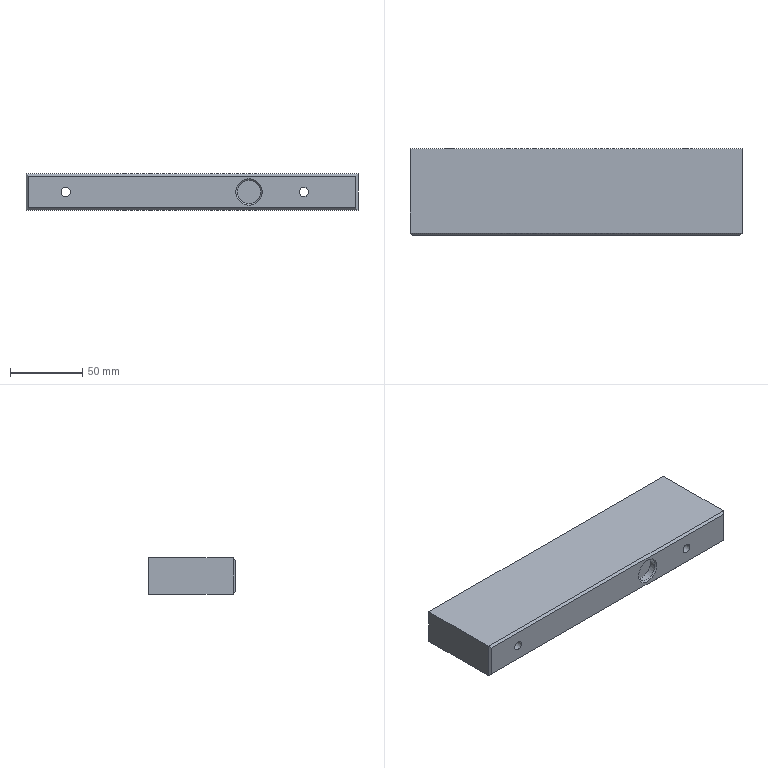CAM job | NX | 3+2 milling, drilling | part box 230 x 60 x 25 mm | stock box 240 x 65.5 x 25 mm
Tools:
number,name,description,diameter,corner_radius,flute_length,length,flutes
1,D16CU,Milling Tool-5 Parameters,16.0,0.0,50.0,75.0,2
3,D8点钻,Chamfer Mill,8.0,0.0,50.0,75.0,2
2,D16.,Milling Tool-5 Parameters,16.0,0.0,50.0,75.0,2
20,D63精,Milling Tool-5 Parameters,63.0,0.0,50.0,75.0,2
18,D63粗,Milling Tool-5 Parameters,63.0,0.0,50.0,75.0,2
19,4倒角,Drilling Tool,4.0,0.0,35.0,50.0,2
21,Z6.5,Drilling Tool,6.5,0.0,35.0,50.0,2
24,D10.,Milling Tool-5 Parameters,10.0,0.0,30.0,30.0,4
9,Z5.,Drilling Tool,5.0,0.0,35.0,50.0,2
Operations:
program,operation,operation_type,tool,method,geometry_group,spindle_rpm,surface_speed,feed_per_tooth,feed_cut,feed_plunge,cut_length_mm,path_length_mm,cut_time_min,machine_time_min
G54,FLOOR_FACING_COPY_2_1,VolumeBased25DMillingOperation,D63粗,METHOD,WORKPIECE,1600.0,316.0,0.3125,1000.0,100.0,319.0,412.8,0.319,0.3284
G54,ADAPTIVE_MILLING,CavityMilling,D16CU,METHOD,WORKPIECE,3000.0,150.0,0.5,3000.0,100.0,7277.595,8200.813,2.04,2.132
G54,PLANAR_MILL_COPY,PlanarMilling,D8点钻,METHOD,WORKPIECE,4500.0,113.0,0.0889,800.0,100.0,599.181,704.181,0.749,0.7595
G54,PLANAR_MILL_COPY_COPY_1,PlanarMilling,4倒角,METHOD,WORKPIECE,4500.0,113.0,0.0889,800.0,100.0,594.06,697.66,0.7426,0.7529
G54,PLANAR_MILL,PlanarMilling,D16.,METHOD,WORKPIECE,1300.0,65.0,0.1538,400.0,100.0,1273.429,1424.429,3.184,3.199
G54,FLOOR_FACING_COPY_2_1_COPY,VolumeBased25DMillingOperation,D63精,METHOD,WORKPIECE,1600.0,316.0,0.125,400.0,100.0,319.0,413.0,0.7975,0.8069
反面,FLOOR_FACING_COPY_2_1_COPY_1,VolumeBased25DMillingOperation,D63粗,METHOD,WORKPIECE,1600.0,316.0,0.3125,1000.0,100.0,5742.0,11227.0,5.742,6.29
反面,FLOOR_FACING_COPY_2_1_COPY_COPY,VolumeBased25DMillingOperation,D63精,METHOD,WORKPIECE,1600.0,316.0,0.1562,500.0,100.0,319.0,413.0,0.638,0.6474
反面,FLOOR_FACING_COPY_2_1_COPY_COPY_COPY,VolumeBased25DMillingOperation,D63精,METHOD,WORKPIECE,1600.0,316.0,0.1562,500.0,100.0,319.0,413.0,0.638,0.6474
反面,PLANAR_MILL_COPY_COPY,PlanarMilling,D8点钻,METHOD,WORKPIECE,4500.0,113.0,0.1333,1200.0,100.0,598.543,703.543,0.4988,0.5093
反面,PLANAR_MILL_COPY_COPY_1_COPY,PlanarMilling,4倒角,METHOD,WORKPIECE,4500.0,113.0,0.0889,800.0,100.0,594.06,697.66,0.7426,0.7529
SIDE,SPOT_FACING,Operation,D8点钻,METHOD,WORKPIECE_1,1500.0,37.0,0.0333,100.0,0.0,16.2,261.468,0.162,0.1865
SIDE,PECK_DRILLING_COPY_1,Operation,Z5.,METHOD,WORKPIECE_1,2500.0,39.0,0.026,130.0,0.0,66.0,360.027,0.5077,0.5371
SIDE,PECK_DRILLING,Operation,Z6.5,METHOD,WORKPIECE_1,1200.0,19.0,0.0333,80.0,0.0,136.0,500.027,1.7,1.736
SIDE,PECK_DRILLING_COPY,Operation,Z6.5,METHOD,WORKPIECE_1,1200.0,19.0,0.0333,80.0,0.0,8.5,77.0,0.1062,0.1131
SIDE,HOLE_MILLING,CylinderMilling,D10.,METHOD,WORKPIECE_1,2800.0,87.0,0.0714,800.0,100.0,605.717,670.697,0.7571,0.7636
SIDE,HOLE_MILLING_COPY,CylinderMilling,D10.,METHOD,WORKPIECE_1,2500.0,78.0,0.015,150.0,100.0,29.217,100.217,0.1948,0.2019
SIDE,PLANAR_MILL_1,PlanarMilling,D8点钻,METHOD,WORKPIECE_1,4500.0,113.0,0.0333,300.0,100.0,53.354,111.354,0.1778,0.1836
SIDE,PLANAR_MILL_1_COPY,PlanarMilling,4倒角,METHOD,WORKPIECE_1,4500.0,113.0,0.0333,300.0,100.0,55.867,113.267,0.1862,0.192